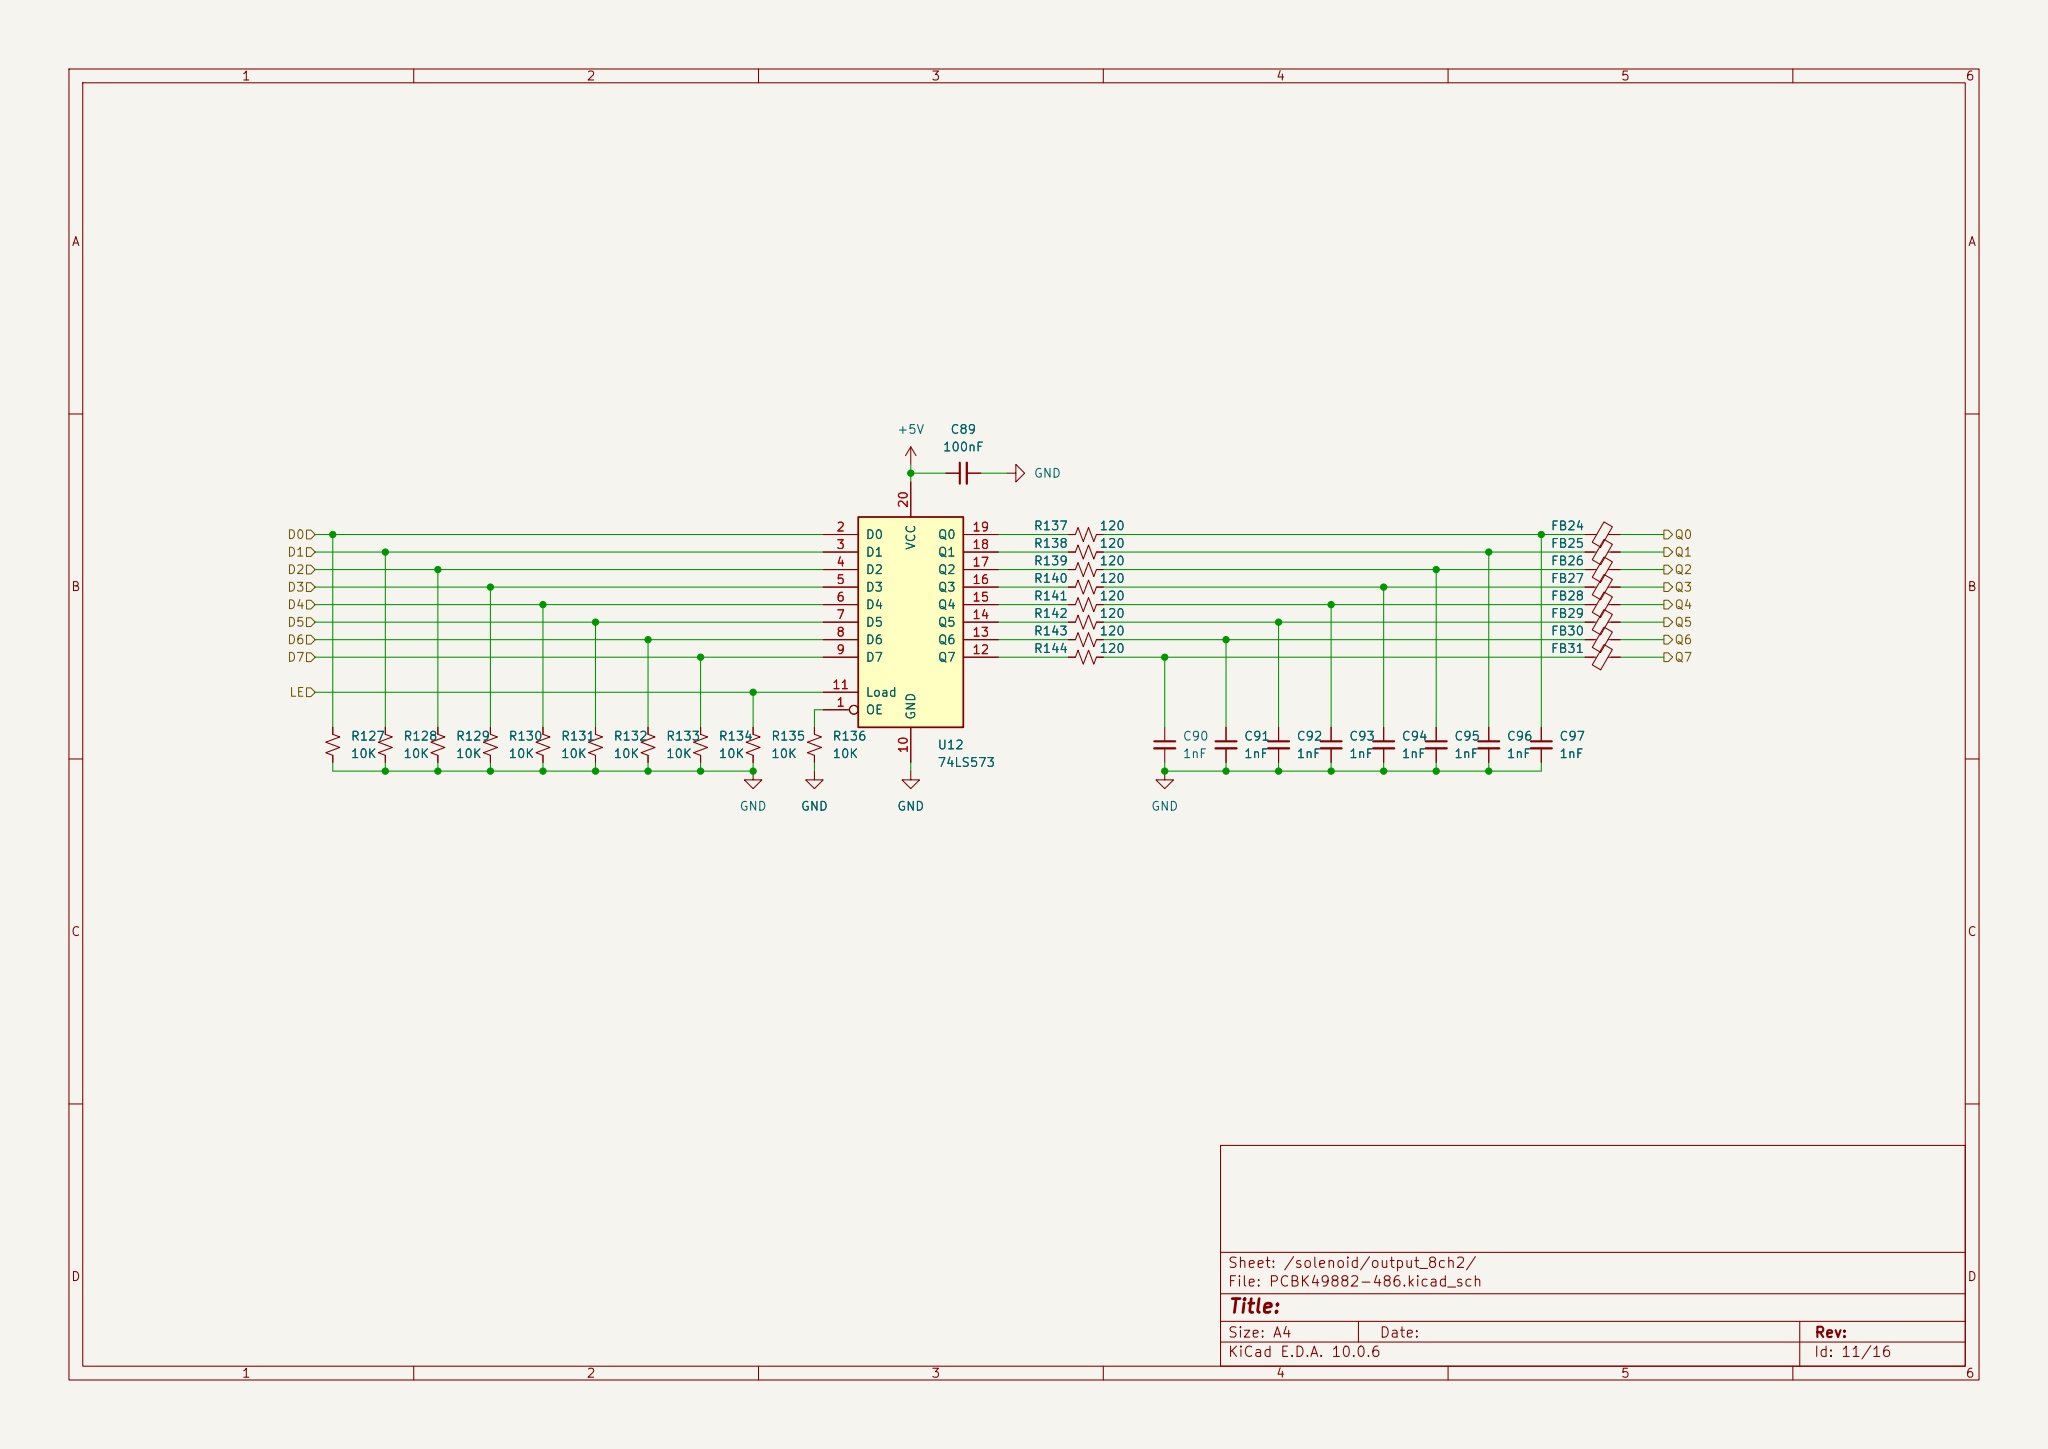Circuit board | KiCad | 536 parts | 438 nets | one sheet of the schematic
Parts on this sheet (reference | value | footprint):
C89 | 100nF | Capacitor_SMD:C_0603_1608Metric
C90
C91
C92
C93
C94
C95
C96
C97
FB24
FB25
FB26
FB27
FB28
FB29
FB30
FB31
R127
R128
R129
R130
R131
R132
R133
R134
R135
R136
R137
R138
R139
R140
R141
R142
R143
R144
U12
Nets of these parts (net: part-pin ...):
+5V: C89-1 U12-20
/core_board_b2b/PA0_C{slash}ADC12_INP0: R127-1 U12-2
/core_board_b2b/PA1_C{slash}ADC12_INP1: R128-1 U12-3
/core_board_b2b/PA3{slash}ADC12_INP15: R131-1 U12-6
/core_board_b2b/PA4{slash}ADC12_INP18: R132-1 U12-7
/core_board_b2b/PA5{slash}ADC12_INP19: R133-1 U12-8
/core_board_b2b/PA6{slash}ADC12_INP3: R134-1 U12-9
/core_board_b2b/PC2_C{slash}ADC3_INP0: R129-1 U12-4
/core_board_b2b/PC3_C{slash}ADC3_INP1: R130-1 U12-5
/core_board_b2b/PF10{slash}ADC3_INP6: R135-1 U12-11
/solenoid/OUTPUT16: FB24-2
/solenoid/OUTPUT17: FB25-2
/solenoid/OUTPUT18: FB26-2
/solenoid/OUTPUT19: FB27-2
/solenoid/OUTPUT20: FB28-2
/solenoid/OUTPUT21: FB29-2
/solenoid/OUTPUT22: FB30-2
/solenoid/OUTPUT23: FB31-2
GND: C89-2 C90-2 C91-2 C92-2 C93-2 C94-2 C95-2 C96-2 C97-2 R127-2 R128-2 R129-2 R130-2 R131-2 R132-2 R133-2 R134-2 R135-2 R136-2 U12-10
Net-(C90-Pad1): C90-1 FB31-1 R144-2
Net-(C91-Pad1): C91-1 FB30-1 R143-2
Net-(C92-Pad1): C92-1 FB29-1 R142-2
Net-(C93-Pad1): C93-1 FB28-1 R141-2
Net-(C94-Pad1): C94-1 FB27-1 R140-2
Net-(C95-Pad1): C95-1 FB26-1 R139-2
Net-(C96-Pad1): C96-1 FB25-1 R138-2
Net-(C97-Pad1): C97-1 FB24-1 R137-2
Net-(U12-OE): R136-1 U12-1
Net-(U12-Q0): R137-1 U12-19
Net-(U12-Q1): R138-1 U12-18
Net-(U12-Q2): R139-1 U12-17
Net-(U12-Q3): R140-1 U12-16
Net-(U12-Q4): R141-1 U12-15
Net-(U12-Q5): R142-1 U12-14
Net-(U12-Q6): R143-1 U12-13
Net-(U12-Q7): R144-1 U12-12